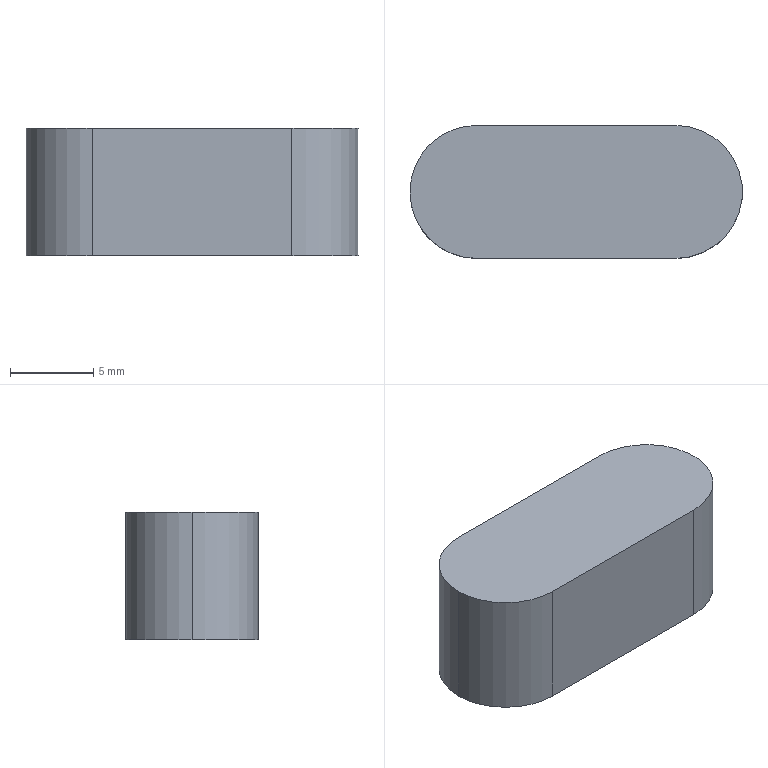Part | STEP file | Keyway 8x20V11_Default<Machined> | 1 solid | 7 faces | box 20 x 8 x 7.7 mm | volume 1126 mm3 | plane 4 | cylinder 3 | commonest cylinder face diameters 8 x3
STEP:
#1=CARTESIAN_POINT('',(0.,0.,0.));
#2=DIRECTION('',(0.,0.,1.));
#3=DIRECTION('',(1.,0.,0.));
#4=AXIS2_PLACEMENT_3D('',#1,#2,#3);
#5=CARTESIAN_POINT('',(-16.,0.,7.7));
#6=VERTEX_POINT('',#5);
#7=CARTESIAN_POINT('',(-12.,-4.,7.7));
#8=VERTEX_POINT('',#7);
#9=CARTESIAN_POINT('',(-12.,0.,7.7));
#10=DIRECTION('',(0.,0.,1.));
#11=DIRECTION('',(1.,0.,0.));
#12=AXIS2_PLACEMENT_3D('',#9,#10,#11);
#13=CIRCLE('',#12,4.);
#14=CARTESIAN_POINT('',(-12.,0.,7.7));
#15=DIRECTION('',(0.,0.,-1.));
#16=DIRECTION('',(-1.,0.,0.));
#17=AXIS2_PLACEMENT_3D('',#14,#15,#16);
#18=CYLINDRICAL_SURFACE('',#17,4.);
#19=CARTESIAN_POINT('',(9.425,0.));
#20=DIRECTION('',(-1.,0.));
#21=VECTOR('',#20,1.);
#22=LINE('',#19,#21);
#23=(GEOMETRIC_REPRESENTATION_CONTEXT(2)PARAMETRIC_REPRESENTATION_CONTEXT()REPRESENTATION_CONTEXT('',''));
#24=DEFINITIONAL_REPRESENTATION('',(#22),#23);
#25=PCURVE('',#18,#24);
#26=CARTESIAN_POINT('',(0.,0.,7.7));
#27=DIRECTION('',(0.,0.,1.));
#28=DIRECTION('',(1.,0.,0.));
#29=AXIS2_PLACEMENT_3D('',#26,#27,#28);
#30=PLANE('',#29);
#31=CARTESIAN_POINT('',(-12.,0.));
#32=DIRECTION('',(1.,0.));
#33=AXIS2_PLACEMENT_2D('',#31,#32);
#34=CIRCLE('',#33,4.);
#35=(GEOMETRIC_REPRESENTATION_CONTEXT(2)PARAMETRIC_REPRESENTATION_CONTEXT()REPRESENTATION_CONTEXT('',''));
#36=DEFINITIONAL_REPRESENTATION('',(#34),#35);
#37=PCURVE('',#30,#36);
#38=SURFACE_CURVE('',#13,(#25,#37),.PCURVE_S1.);
#39=EDGE_CURVE('',#6,#8,#38,.T.);
#40=ORIENTED_EDGE('',*,*,#39,.F.);
#41=CARTESIAN_POINT('',(-16.,0.,0.));
#42=VERTEX_POINT('',#41);
#43=CARTESIAN_POINT('',(-16.,0.,7.7));
#44=DIRECTION('',(0.,0.,-1.));
#45=VECTOR('',#44,1.);
#46=LINE('',#43,#45);
#47=CARTESIAN_POINT('',(6.283,0.));
#48=DIRECTION('',(0.,1.));
#49=VECTOR('',#48,1.);
#50=LINE('',#47,#49);
#51=(GEOMETRIC_REPRESENTATION_CONTEXT(2)PARAMETRIC_REPRESENTATION_CONTEXT()REPRESENTATION_CONTEXT('',''));
#52=DEFINITIONAL_REPRESENTATION('',(#50),#51);
#53=PCURVE('',#18,#52);
#54=CARTESIAN_POINT('',(-12.,0.,7.7));
#55=DIRECTION('',(0.,0.,-1.));
#56=DIRECTION('',(-1.,0.,0.));
#57=AXIS2_PLACEMENT_3D('',#54,#55,#56);
#58=CYLINDRICAL_SURFACE('',#57,4.);
#59=CARTESIAN_POINT('',(0.,0.));
#60=DIRECTION('',(0.,1.));
#61=VECTOR('',#60,1.);
#62=LINE('',#59,#61);
#63=(GEOMETRIC_REPRESENTATION_CONTEXT(2)PARAMETRIC_REPRESENTATION_CONTEXT()REPRESENTATION_CONTEXT('',''));
#64=DEFINITIONAL_REPRESENTATION('',(#62),#63);
#65=PCURVE('',#58,#64);
#66=SURFACE_CURVE('',#46,(#53,#65),.PCURVE_S1.);
#67=EDGE_CURVE('',#6,#42,#66,.T.);
#68=ORIENTED_EDGE('',*,*,#67,.T.);
#69=CARTESIAN_POINT('',(-12.,-4.,0.));
#70=VERTEX_POINT('',#69);
#71=CARTESIAN_POINT('',(-12.,0.,0.));
#72=DIRECTION('',(0.,0.,1.));
#73=DIRECTION('',(1.,0.,0.));
#74=AXIS2_PLACEMENT_3D('',#71,#72,#73);
#75=CIRCLE('',#74,4.);
#76=CARTESIAN_POINT('',(9.425,7.7));
#77=DIRECTION('',(-1.,0.));
#78=VECTOR('',#77,1.);
#79=LINE('',#76,#78);
#80=(GEOMETRIC_REPRESENTATION_CONTEXT(2)PARAMETRIC_REPRESENTATION_CONTEXT()REPRESENTATION_CONTEXT('',''));
#81=DEFINITIONAL_REPRESENTATION('',(#79),#80);
#82=PCURVE('',#18,#81);
#83=CARTESIAN_POINT('',(0.,0.,0.));
#84=DIRECTION('',(0.,0.,1.));
#85=DIRECTION('',(1.,0.,0.));
#86=AXIS2_PLACEMENT_3D('',#83,#84,#85);
#87=PLANE('',#86);
#88=CARTESIAN_POINT('',(-12.,0.));
#89=DIRECTION('',(1.,0.));
#90=AXIS2_PLACEMENT_2D('',#88,#89);
#91=CIRCLE('',#90,4.);
#92=(GEOMETRIC_REPRESENTATION_CONTEXT(2)PARAMETRIC_REPRESENTATION_CONTEXT()REPRESENTATION_CONTEXT('',''));
#93=DEFINITIONAL_REPRESENTATION('',(#91),#92);
#94=PCURVE('',#87,#93);
#95=SURFACE_CURVE('',#75,(#82,#94),.PCURVE_S1.);
#96=EDGE_CURVE('',#42,#70,#95,.T.);
#97=ORIENTED_EDGE('',*,*,#96,.T.);
#98=CARTESIAN_POINT('',(-12.,-4.,7.7));
#99=DIRECTION('',(0.,0.,-1.));
#100=VECTOR('',#99,1.);
#101=LINE('',#98,#100);
#102=CARTESIAN_POINT('',(4.712,0.));
#103=DIRECTION('',(0.,1.));
#104=VECTOR('',#103,1.);
#105=LINE('',#102,#104);
#106=(GEOMETRIC_REPRESENTATION_CONTEXT(2)PARAMETRIC_REPRESENTATION_CONTEXT()REPRESENTATION_CONTEXT('',''));
#107=DEFINITIONAL_REPRESENTATION('',(#105),#106);
#108=PCURVE('',#18,#107);
#109=CARTESIAN_POINT('',(0.,-4.,7.7));
#110=DIRECTION('',(0.,1.,0.));
#111=DIRECTION('',(-1.,0.,0.));
#112=AXIS2_PLACEMENT_3D('',#109,#110,#111);
#113=PLANE('',#112);
#114=CARTESIAN_POINT('',(12.,0.));
#115=DIRECTION('',(0.,-1.));
#116=VECTOR('',#115,1.);
#117=LINE('',#114,#116);
#118=(GEOMETRIC_REPRESENTATION_CONTEXT(2)PARAMETRIC_REPRESENTATION_CONTEXT()REPRESENTATION_CONTEXT('',''));
#119=DEFINITIONAL_REPRESENTATION('',(#117),#118);
#120=PCURVE('',#113,#119);
#121=SURFACE_CURVE('',#101,(#108,#120),.PCURVE_S1.);
#122=EDGE_CURVE('',#8,#70,#121,.T.);
#123=ORIENTED_EDGE('',*,*,#122,.F.);
#124=EDGE_LOOP('',(#40,#68,#97,#123));
#125=FACE_BOUND('',#124,.T.);
#126=ADVANCED_FACE('',(#125),#18,.T.);
#127=CARTESIAN_POINT('',(0.,-4.,0.));
#128=VERTEX_POINT('',#127);
#129=CARTESIAN_POINT('',(0.,4.,0.));
#130=VERTEX_POINT('',#129);
#131=CARTESIAN_POINT('',(0.,0.,0.));
#132=DIRECTION('',(0.,0.,1.));
#133=DIRECTION('',(1.,0.,0.));
#134=AXIS2_PLACEMENT_3D('',#131,#132,#133);
#135=CIRCLE('',#134,4.);
#136=CARTESIAN_POINT('',(0.,0.,7.7));
#137=DIRECTION('',(0.,0.,-1.));
#138=DIRECTION('',(-1.,0.,0.));
#139=AXIS2_PLACEMENT_3D('',#136,#137,#138);
#140=CYLINDRICAL_SURFACE('',#139,4.);
#141=CARTESIAN_POINT('',(9.425,7.7));
#142=DIRECTION('',(-1.,0.));
#143=VECTOR('',#142,1.);
#144=LINE('',#141,#143);
#145=(GEOMETRIC_REPRESENTATION_CONTEXT(2)PARAMETRIC_REPRESENTATION_CONTEXT()REPRESENTATION_CONTEXT('',''));
#146=DEFINITIONAL_REPRESENTATION('',(#144),#145);
#147=PCURVE('',#140,#146);
#148=CARTESIAN_POINT('',(0.,0.));
#149=DIRECTION('',(1.,0.));
#150=AXIS2_PLACEMENT_2D('',#148,#149);
#151=CIRCLE('',#150,4.);
#152=(GEOMETRIC_REPRESENTATION_CONTEXT(2)PARAMETRIC_REPRESENTATION_CONTEXT()REPRESENTATION_CONTEXT('',''));
#153=DEFINITIONAL_REPRESENTATION('',(#151),#152);
#154=PCURVE('',#87,#153);
#155=SURFACE_CURVE('',#135,(#147,#154),.PCURVE_S1.);
#156=EDGE_CURVE('',#128,#130,#155,.T.);
#157=ORIENTED_EDGE('',*,*,#156,.T.);
#158=CARTESIAN_POINT('',(0.,4.,7.7));
#159=VERTEX_POINT('',#158);
#160=CARTESIAN_POINT('',(0.,4.,7.7));
#161=DIRECTION('',(0.,0.,-1.));
#162=VECTOR('',#161,1.);
#163=LINE('',#160,#162);
#164=CARTESIAN_POINT('',(1.571,0.));
#165=DIRECTION('',(0.,1.));
#166=VECTOR('',#165,1.);
#167=LINE('',#164,#166);
#168=(GEOMETRIC_REPRESENTATION_CONTEXT(2)PARAMETRIC_REPRESENTATION_CONTEXT()REPRESENTATION_CONTEXT('',''));
#169=DEFINITIONAL_REPRESENTATION('',(#167),#168);
#170=PCURVE('',#140,#169);
#171=CARTESIAN_POINT('',(0.,4.,7.7));
#172=DIRECTION('',(0.,-1.,0.));
#173=DIRECTION('',(1.,0.,0.));
#174=AXIS2_PLACEMENT_3D('',#171,#172,#173);
#175=PLANE('',#174);
#176=CARTESIAN_POINT('',(0.,0.));
#177=DIRECTION('',(0.,-1.));
#178=VECTOR('',#177,1.);
#179=LINE('',#176,#178);
#180=(GEOMETRIC_REPRESENTATION_CONTEXT(2)PARAMETRIC_REPRESENTATION_CONTEXT()REPRESENTATION_CONTEXT('',''));
#181=DEFINITIONAL_REPRESENTATION('',(#179),#180);
#182=PCURVE('',#175,#181);
#183=SURFACE_CURVE('',#163,(#170,#182),.PCURVE_S1.);
#184=EDGE_CURVE('',#159,#130,#183,.T.);
#185=ORIENTED_EDGE('',*,*,#184,.F.);
#186=CARTESIAN_POINT('',(0.,-4.,7.7));
#187=VERTEX_POINT('',#186);
#188=CARTESIAN_POINT('',(0.,0.,7.7));
#189=DIRECTION('',(0.,0.,1.));
#190=DIRECTION('',(1.,0.,0.));
#191=AXIS2_PLACEMENT_3D('',#188,#189,#190);
#192=CIRCLE('',#191,4.);
#193=CARTESIAN_POINT('',(9.425,0.));
#194=DIRECTION('',(-1.,0.));
#195=VECTOR('',#194,1.);
#196=LINE('',#193,#195);
#197=(GEOMETRIC_REPRESENTATION_CONTEXT(2)PARAMETRIC_REPRESENTATION_CONTEXT()REPRESENTATION_CONTEXT('',''));
#198=DEFINITIONAL_REPRESENTATION('',(#196),#197);
#199=PCURVE('',#140,#198);
#200=CARTESIAN_POINT('',(0.,0.));
#201=DIRECTION('',(1.,0.));
#202=AXIS2_PLACEMENT_2D('',#200,#201);
#203=CIRCLE('',#202,4.);
#204=(GEOMETRIC_REPRESENTATION_CONTEXT(2)PARAMETRIC_REPRESENTATION_CONTEXT()REPRESENTATION_CONTEXT('',''));
#205=DEFINITIONAL_REPRESENTATION('',(#203),#204);
#206=PCURVE('',#30,#205);
#207=SURFACE_CURVE('',#192,(#199,#206),.PCURVE_S1.);
#208=EDGE_CURVE('',#187,#159,#207,.T.);
#209=ORIENTED_EDGE('',*,*,#208,.F.);
#210=CARTESIAN_POINT('',(0.,-4.,7.7));
#211=DIRECTION('',(0.,0.,-1.));
#212=VECTOR('',#211,1.);
#213=LINE('',#210,#212);
#214=CARTESIAN_POINT('',(4.712,0.));
#215=DIRECTION('',(0.,1.));
#216=VECTOR('',#215,1.);
#217=LINE('',#214,#216);
#218=(GEOMETRIC_REPRESENTATION_CONTEXT(2)PARAMETRIC_REPRESENTATION_CONTEXT()REPRESENTATION_CONTEXT('',''));
#219=DEFINITIONAL_REPRESENTATION('',(#217),#218);
#220=PCURVE('',#140,#219);
#221=CARTESIAN_POINT('',(0.,0.));
#222=DIRECTION('',(0.,-1.));
#223=VECTOR('',#222,1.);
#224=LINE('',#221,#223);
#225=(GEOMETRIC_REPRESENTATION_CONTEXT(2)PARAMETRIC_REPRESENTATION_CONTEXT()REPRESENTATION_CONTEXT('',''));
#226=DEFINITIONAL_REPRESENTATION('',(#224),#225);
#227=PCURVE('',#113,#226);
#228=SURFACE_CURVE('',#213,(#220,#227),.PCURVE_S1.);
#229=EDGE_CURVE('',#187,#128,#228,.T.);
#230=ORIENTED_EDGE('',*,*,#229,.T.);
#231=EDGE_LOOP('',(#157,#185,#209,#230));
#232=FACE_BOUND('',#231,.T.);
#233=ADVANCED_FACE('',(#232),#140,.T.);
#234=CARTESIAN_POINT('',(-12.,4.,0.));
#235=VERTEX_POINT('',#234);
#236=CARTESIAN_POINT('',(0.,4.,0.));
#237=DIRECTION('',(-1.,0.,0.));
#238=VECTOR('',#237,1.);
#239=LINE('',#236,#238);
#240=CARTESIAN_POINT('',(0.,-7.7));
#241=DIRECTION('',(-1.,0.));
#242=VECTOR('',#241,1.);
#243=LINE('',#240,#242);
#244=(GEOMETRIC_REPRESENTATION_CONTEXT(2)PARAMETRIC_REPRESENTATION_CONTEXT()REPRESENTATION_CONTEXT('',''));
#245=DEFINITIONAL_REPRESENTATION('',(#243),#244);
#246=PCURVE('',#175,#245);
#247=CARTESIAN_POINT('',(0.,4.));
#248=DIRECTION('',(-1.,0.));
#249=VECTOR('',#248,1.);
#250=LINE('',#247,#249);
#251=(GEOMETRIC_REPRESENTATION_CONTEXT(2)PARAMETRIC_REPRESENTATION_CONTEXT()REPRESENTATION_CONTEXT('',''));
#252=DEFINITIONAL_REPRESENTATION('',(#250),#251);
#253=PCURVE('',#87,#252);
#254=SURFACE_CURVE('',#239,(#246,#253),.PCURVE_S1.);
#255=EDGE_CURVE('',#130,#235,#254,.T.);
#256=ORIENTED_EDGE('',*,*,#255,.T.);
#257=CARTESIAN_POINT('',(-12.,4.,7.7));
#258=VERTEX_POINT('',#257);
#259=CARTESIAN_POINT('',(-12.,4.,7.7));
#260=DIRECTION('',(0.,0.,-1.));
#261=VECTOR('',#260,1.);
#262=LINE('',#259,#261);
#263=CARTESIAN_POINT('',(-12.,0.));
#264=DIRECTION('',(0.,-1.));
#265=VECTOR('',#264,1.);
#266=LINE('',#263,#265);
#267=(GEOMETRIC_REPRESENTATION_CONTEXT(2)PARAMETRIC_REPRESENTATION_CONTEXT()REPRESENTATION_CONTEXT('',''));
#268=DEFINITIONAL_REPRESENTATION('',(#266),#267);
#269=PCURVE('',#175,#268);
#270=CARTESIAN_POINT('',(1.571,0.));
#271=DIRECTION('',(0.,1.));
#272=VECTOR('',#271,1.);
#273=LINE('',#270,#272);
#274=(GEOMETRIC_REPRESENTATION_CONTEXT(2)PARAMETRIC_REPRESENTATION_CONTEXT()REPRESENTATION_CONTEXT('',''));
#275=DEFINITIONAL_REPRESENTATION('',(#273),#274);
#276=PCURVE('',#58,#275);
#277=SURFACE_CURVE('',#262,(#269,#276),.PCURVE_S1.);
#278=EDGE_CURVE('',#258,#235,#277,.T.);
#279=ORIENTED_EDGE('',*,*,#278,.F.);
#280=CARTESIAN_POINT('',(0.,4.,7.7));
#281=DIRECTION('',(-1.,0.,0.));
#282=VECTOR('',#281,1.);
#283=LINE('',#280,#282);
#284=CARTESIAN_POINT('',(0.,0.));
#285=DIRECTION('',(-1.,0.));
#286=VECTOR('',#285,1.);
#287=LINE('',#284,#286);
#288=(GEOMETRIC_REPRESENTATION_CONTEXT(2)PARAMETRIC_REPRESENTATION_CONTEXT()REPRESENTATION_CONTEXT('',''));
#289=DEFINITIONAL_REPRESENTATION('',(#287),#288);
#290=PCURVE('',#175,#289);
#291=CARTESIAN_POINT('',(0.,4.));
#292=DIRECTION('',(-1.,0.));
#293=VECTOR('',#292,1.);
#294=LINE('',#291,#293);
#295=(GEOMETRIC_REPRESENTATION_CONTEXT(2)PARAMETRIC_REPRESENTATION_CONTEXT()REPRESENTATION_CONTEXT('',''));
#296=DEFINITIONAL_REPRESENTATION('',(#294),#295);
#297=PCURVE('',#30,#296);
#298=SURFACE_CURVE('',#283,(#290,#297),.PCURVE_S1.);
#299=EDGE_CURVE('',#159,#258,#298,.T.);
#300=ORIENTED_EDGE('',*,*,#299,.F.);
#301=ORIENTED_EDGE('',*,*,#184,.T.);
#302=EDGE_LOOP('',(#256,#279,#300,#301));
#303=FACE_BOUND('',#302,.T.);
#304=ADVANCED_FACE('',(#303),#175,.F.);
#305=ORIENTED_EDGE('',*,*,#67,.F.);
#306=CARTESIAN_POINT('',(-12.,0.,7.7));
#307=DIRECTION('',(0.,0.,1.));
#308=DIRECTION('',(1.,0.,0.));
#309=AXIS2_PLACEMENT_3D('',#306,#307,#308);
#310=CIRCLE('',#309,4.);
#311=CARTESIAN_POINT('',(3.142,0.));
#312=DIRECTION('',(-1.,0.));
#313=VECTOR('',#312,1.);
#314=LINE('',#311,#313);
#315=(GEOMETRIC_REPRESENTATION_CONTEXT(2)PARAMETRIC_REPRESENTATION_CONTEXT()REPRESENTATION_CONTEXT('',''));
#316=DEFINITIONAL_REPRESENTATION('',(#314),#315);
#317=PCURVE('',#58,#316);
#318=CARTESIAN_POINT('',(-12.,0.));
#319=DIRECTION('',(1.,0.));
#320=AXIS2_PLACEMENT_2D('',#318,#319);
#321=CIRCLE('',#320,4.);
#322=(GEOMETRIC_REPRESENTATION_CONTEXT(2)PARAMETRIC_REPRESENTATION_CONTEXT()REPRESENTATION_CONTEXT('',''));
#323=DEFINITIONAL_REPRESENTATION('',(#321),#322);
#324=PCURVE('',#30,#323);
#325=SURFACE_CURVE('',#310,(#317,#324),.PCURVE_S1.);
#326=EDGE_CURVE('',#258,#6,#325,.T.);
#327=ORIENTED_EDGE('',*,*,#326,.F.);
#328=ORIENTED_EDGE('',*,*,#278,.T.);
#329=CARTESIAN_POINT('',(-12.,0.,0.));
#330=DIRECTION('',(0.,0.,1.));
#331=DIRECTION('',(1.,0.,0.));
#332=AXIS2_PLACEMENT_3D('',#329,#330,#331);
#333=CIRCLE('',#332,4.);
#334=CARTESIAN_POINT('',(3.142,7.7));
#335=DIRECTION('',(-1.,0.));
#336=VECTOR('',#335,1.);
#337=LINE('',#334,#336);
#338=(GEOMETRIC_REPRESENTATION_CONTEXT(2)PARAMETRIC_REPRESENTATION_CONTEXT()REPRESENTATION_CONTEXT('',''));
#339=DEFINITIONAL_REPRESENTATION('',(#337),#338);
#340=PCURVE('',#58,#339);
#341=CARTESIAN_POINT('',(-12.,0.));
#342=DIRECTION('',(1.,0.));
#343=AXIS2_PLACEMENT_2D('',#341,#342);
#344=CIRCLE('',#343,4.);
#345=(GEOMETRIC_REPRESENTATION_CONTEXT(2)PARAMETRIC_REPRESENTATION_CONTEXT()REPRESENTATION_CONTEXT('',''));
#346=DEFINITIONAL_REPRESENTATION('',(#344),#345);
#347=PCURVE('',#87,#346);
#348=SURFACE_CURVE('',#333,(#340,#347),.PCURVE_S1.);
#349=EDGE_CURVE('',#235,#42,#348,.T.);
#350=ORIENTED_EDGE('',*,*,#349,.T.);
#351=EDGE_LOOP('',(#305,#327,#328,#350));
#352=FACE_BOUND('',#351,.T.);
#353=ADVANCED_FACE('',(#352),#58,.T.);
#354=CARTESIAN_POINT('',(0.,-4.,0.));
#355=DIRECTION('',(1.,0.,0.));
#356=VECTOR('',#355,1.);
#357=LINE('',#354,#356);
#358=CARTESIAN_POINT('',(0.,-7.7));
#359=DIRECTION('',(-1.,0.));
#360=VECTOR('',#359,1.);
#361=LINE('',#358,#360);
#362=(GEOMETRIC_REPRESENTATION_CONTEXT(2)PARAMETRIC_REPRESENTATION_CONTEXT()REPRESENTATION_CONTEXT('',''));
#363=DEFINITIONAL_REPRESENTATION('',(#361),#362);
#364=PCURVE('',#113,#363);
#365=CARTESIAN_POINT('',(0.,-4.));
#366=DIRECTION('',(1.,0.));
#367=VECTOR('',#366,1.);
#368=LINE('',#365,#367);
#369=(GEOMETRIC_REPRESENTATION_CONTEXT(2)PARAMETRIC_REPRESENTATION_CONTEXT()REPRESENTATION_CONTEXT('',''));
#370=DEFINITIONAL_REPRESENTATION('',(#368),#369);
#371=PCURVE('',#87,#370);
#372=SURFACE_CURVE('',#357,(#364,#371),.PCURVE_S1.);
#373=EDGE_CURVE('',#70,#128,#372,.T.);
#374=ORIENTED_EDGE('',*,*,#373,.T.);
#375=ORIENTED_EDGE('',*,*,#229,.F.);
#376=CARTESIAN_POINT('',(0.,-4.,7.7));
#377=DIRECTION('',(1.,0.,0.));
#378=VECTOR('',#377,1.);
#379=LINE('',#376,#378);
#380=CARTESIAN_POINT('',(0.,0.));
#381=DIRECTION('',(-1.,0.));
#382=VECTOR('',#381,1.);
#383=LINE('',#380,#382);
#384=(GEOMETRIC_REPRESENTATION_CONTEXT(2)PARAMETRIC_REPRESENTATION_CONTEXT()REPRESENTATION_CONTEXT('',''));
#385=DEFINITIONAL_REPRESENTATION('',(#383),#384);
#386=PCURVE('',#113,#385);
#387=CARTESIAN_POINT('',(0.,-4.));
#388=DIRECTION('',(1.,0.));
#389=VECTOR('',#388,1.);
#390=LINE('',#387,#389);
#391=(GEOMETRIC_REPRESENTATION_CONTEXT(2)PARAMETRIC_REPRESENTATION_CONTEXT()REPRESENTATION_CONTEXT('',''));
#392=DEFINITIONAL_REPRESENTATION('',(#390),#391);
#393=PCURVE('',#30,#392);
#394=SURFACE_CURVE('',#379,(#386,#393),.PCURVE_S1.);
#395=EDGE_CURVE('',#8,#187,#394,.T.);
#396=ORIENTED_EDGE('',*,*,#395,.F.);
#397=ORIENTED_EDGE('',*,*,#122,.T.);
#398=EDGE_LOOP('',(#374,#375,#396,#397));
#399=FACE_BOUND('',#398,.T.);
#400=ADVANCED_FACE('',(#399),#113,.F.);
#401=ORIENTED_EDGE('',*,*,#208,.T.);
#402=ORIENTED_EDGE('',*,*,#299,.T.);
#403=ORIENTED_EDGE('',*,*,#326,.T.);
#404=ORIENTED_EDGE('',*,*,#39,.T.);
#405=ORIENTED_EDGE('',*,*,#395,.T.);
#406=EDGE_LOOP('',(#401,#402,#403,#404,#405));
#407=FACE_BOUND('',#406,.T.);
#408=ADVANCED_FACE('',(#407),#30,.T.);
#409=ORIENTED_EDGE('',*,*,#156,.F.);
#410=ORIENTED_EDGE('',*,*,#373,.F.);
#411=ORIENTED_EDGE('',*,*,#96,.F.);
#412=ORIENTED_EDGE('',*,*,#349,.F.);
#413=ORIENTED_EDGE('',*,*,#255,.F.);
#414=EDGE_LOOP('',(#409,#410,#411,#412,#413));
#415=FACE_BOUND('',#414,.T.);
#416=ADVANCED_FACE('',(#415),#87,.F.);
#417=CLOSED_SHELL('',(#126,#233,#304,#353,#400,#408,#416));
#418=MANIFOLD_SOLID_BREP('',#417);
#419=(LENGTH_UNIT()NAMED_UNIT(*)SI_UNIT(.MILLI.,.METRE.));
#420=UNCERTAINTY_MEASURE_WITH_UNIT(LENGTH_MEASURE(0.0000001),#419,'','');
#421=(NAMED_UNIT(*)PLANE_ANGLE_UNIT()SI_UNIT($,.RADIAN.));
#422=(NAMED_UNIT(*)SI_UNIT($,.STERADIAN.)SOLID_ANGLE_UNIT());
#423=(GEOMETRIC_REPRESENTATION_CONTEXT(3)GLOBAL_UNCERTAINTY_ASSIGNED_CONTEXT((#420))GLOBAL_UNIT_ASSIGNED_CONTEXT((#419,#421,#422))REPRESENTATION_CONTEXT('',''));
#424=ADVANCED_BREP_SHAPE_REPRESENTATION('',(#4,#418),#423);